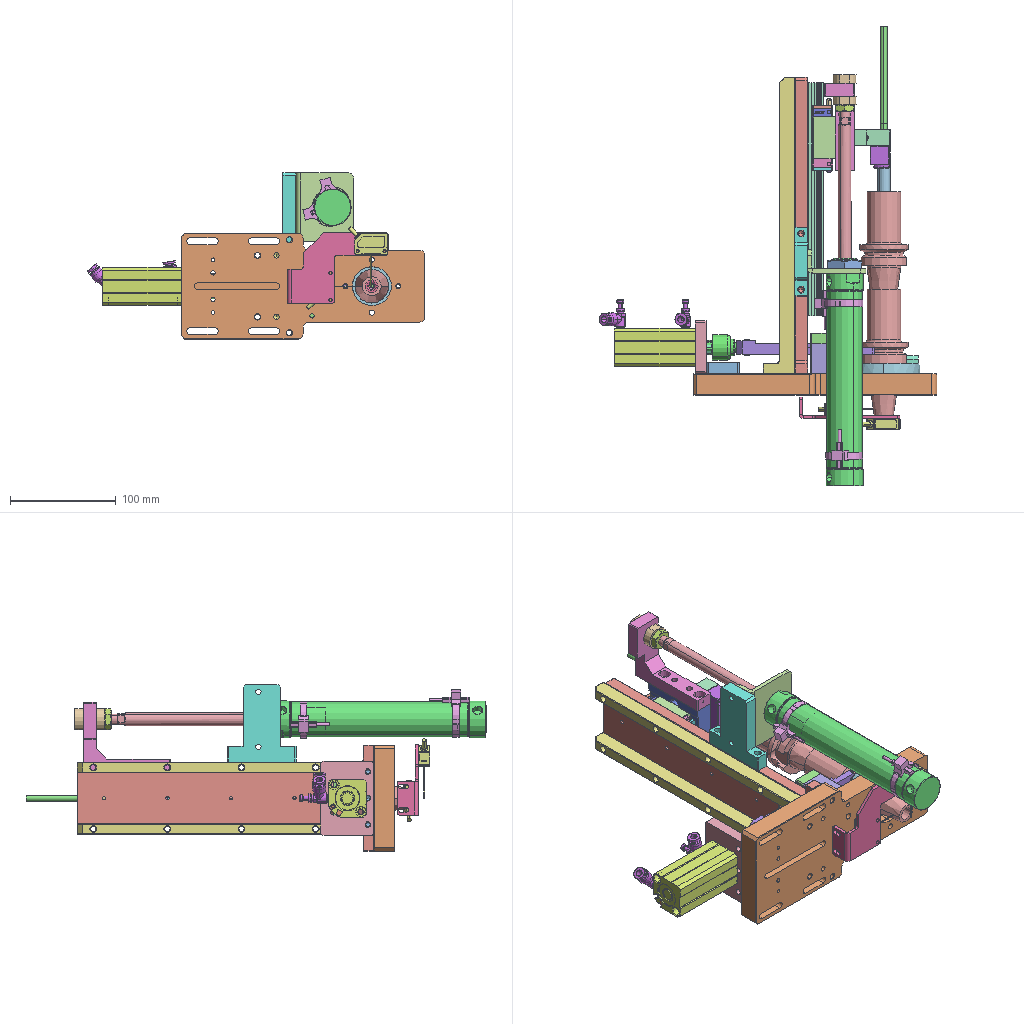Assembly | SolidWorks | 30 different items | 37 placed | box 319 x 435 x 157 mm
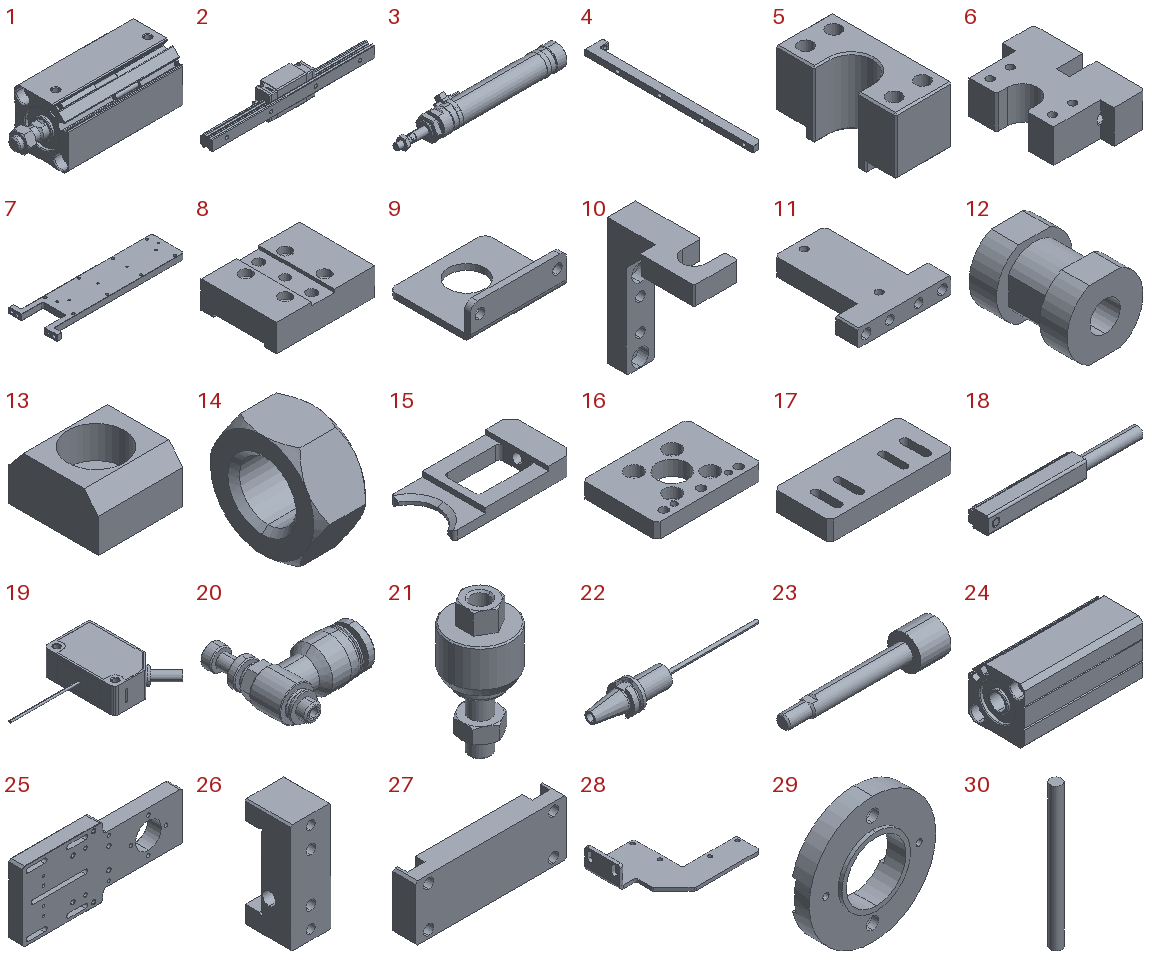Parts list (item | name | quantity | parent item | size | volume | features):
1 | (subassembly) | x1 | - | 95 x 36 x 36 mm | 77347 mm3 | -
2 | (subassembly) | x1 | - | 220 x 28 x 34 mm | 77398 mm3 | features AEMSimFeature 1
3 | (subassembly) | x1 | - | 263.352 x 41.739 x 46.528 mm | 110258 mm3 | features AEMSimFeature 1
4 | - | x2 | - | 30 x 280 x 10 mm | 40714 mm3 | features HoleWzd 3, Chamfer 2, Extrusion 1, Fillet 1, ICE 1
5 | - | x1 | - | 18 x 38 x 21 mm | 8331 mm3 | features Chamfer 1, Cut 1, Extrusion 1, HoleWzd 1, ICE 1
6 | - | x1 | - | 35 x 50 x 15 mm | 18159 mm3 | features HoleWzd 3, Chamfer 2, ICE 2, Cut 1, Extrusion 1
7 | - | x1 | - | 280 x 100 x 12 mm | 201479 mm3 | features HoleWzd 7, Chamfer 2, Fillet 2, Cut 1, Extrusion 1, ICE 1
8 | - | x1 | - | 65 x 50 x 18 mm | 47739 mm3 | features HoleWzd 6, Cut 3, Extrusion 1
9 | - | x1 | - | 65 x 55 x 22 mm | 16429 mm3 | features EdgeFlange 1, Fillet 1, FlatPattern 1, HoleWzd 1, ICE 1, SMBaseFlange 1, SheetMetal 1
10 | - | x1 | - | 28 x 65.5 x 82 mm | 28684 mm3 | features Chamfer 2, HoleWzd 2, ICE 2, Cut 1, Extrusion 1
11 | - | x1 | - | 65 x 73 x 12 mm | 33602 mm3 | features HoleWzd 3, Chamfer 2, Extrusion 1, ICE 1
12 | - | x1 | - | 22 x 28.5 x 20 mm | 6854 mm3 | features ICE 5, Extrusion 1, HoleWzd 1
13 | - | x2 | - | 15 x 15.8 x 9 mm | 1494 mm3 | features Extrusion 1, HoleWzd 1, ICE 1
14 | - | x1 | in 1 | 6 x 13.856 x 12.003 mm | 523.363 mm3 | features BaseBody 1
15 | - | x2 | - | 85 x 45 x 13 mm | 24143 mm3 | features ICE 6, Chamfer 3, Fillet 3, Extrusion 1, HoleWzd 1
16 | - | x1 | - | 70 x 50 x 10 mm | 27882 mm3 | features HoleWzd 3, Chamfer 1, Extrusion 1, ICE 1
17 | - | x1 | - | 70 x 32 x 11 mm | 21010 mm3 | features HoleWzd 4, Chamfer 1, Extrusion 1
18 | - | x2 | in 1 | 40.5 x 5.8 x 4.4 mm | 628.814 mm3 | features BaseBody 1
19 | - | x2 | - | 56.19 x 38.39 x 11 mm | 6633 mm3 | features BaseBody 1, ICE 1
20 | - | x2 | - | 28.5 x 30 x 12.5 mm | 2576 mm3 | features BaseBody 1
21 | - | x1 | - | 24 x 24 x 51 mm | 10568 mm3 | features BaseBody 1
22 | - | x2 | - | 277 x 46 x 46 mm | 91499 mm3 | features BaseBody 10
23 | - | x1 | in 1 | 91 x 20 x 20 mm | 10940 mm3 | features BaseBody 1
24 | - | x1 | in 1 | 76.5 x 36 x 36 mm | 64626 mm3 | features BaseBody 1
25 | - | x1 | - | 230 x 20 x 100 mm | 331110 mm3 | features HoleWzd 11, Chamfer 3, ICE 2, CirPattern 1, Cut 1, Extrusion 1, Fillet 1
26 | - | x1 | - | 25 x 28.4 x 68 mm | 31309 mm3 | features HoleWzd 3, ICE 2, Chamfer 1, Cut 1, Extrusion 1
27 | - | x1 | - | 68 x 10 x 25 mm | 15689 mm3 | features Chamfer 1, Extrusion 1, HoleWzd 1, ICE 1
28 | - | x1 | - | 95 x 67 x 20 mm | 11356 mm3 | features ICE 3, Chamfer 1, Cut 1, Fillet 1, FlatPattern 1, SMBaseFlange 1, SheetMetal 1
29 | - | x1 | - | 68 x 12 x 68 mm | 26017 mm3 | features ICE 6, HoleWzd 2, Revolution 1
30 | - | x1 | - | 12 x 12 x 150 mm | 16965 mm3 | features Extrusion 1
Mates (type | each side: item.copy, entity, surface, feature):
Coincident | 25.1 face plane Boss-Extrude 1 | 26.1 face plane Boss-Extrude 1
Coincident | 26.1 face plane Boss-Extrude 1 | 27.1 face plane Boss-Extrude 1 | 3 times
Symmetric | 25.1 face plane Boss-Extrude 1 | 25.1 face plane Boss-Extrude 1 | 26.1 plane
DistanceDim | 26.1 face plane Boss-Extrude 1 | 25.1 face plane Boss-Extrude 1
Coincident | 19.1 face plane E-MSMD61N-2M_l-1-solid1 | 28.1 face plane Base-Flange 1
Concentric | 19.1 face cylinder E-MSMD61N-2M_l-1-solid1 | 28.1 face cylinder Cut-Extrude 2 | 2 times
Coincident | 28.1 face plane Base-Flange 1 | 19.2 face plane E-MSMD61N-2M_l-1-solid1
Concentric | 28.1 face cylinder Cut-Extrude 2 | 19.2 face cylinder E-MSMD61N-2M_l-1-solid1 | 2 times
Coincident | 25.1 face plane Boss-Extrude 1 | 29.1 face plane Revolve 1
Concentric | 25.1 face cylinder Cut-Extrude 1 | 29.1 face cylinder Cut-Extrude 1
Coincident | 29.1 face plane Cut-Extrude 6 | 13.1 face plane Boss-Extrude 1
Concentric | 29.1 face cylinder M4 Tapped Hole 1 | 13.1 face cylinder M4 沉头Hole 1
Parallel | 29.1 face plane Cut-Extrude 6 | 13.1 face plane Boss-Extrude 1
Coincident | 29.1 face plane Cut-Extrude 6 | 13.2 face plane Boss-Extrude 1
Concentric | 29.1 face cylinder M4 Tapped Hole 1 | 13.2 face cylinder M4 沉头Hole 1
Parallel | 29.1 face plane Cut-Extrude 6 | 13.2 face plane Boss-Extrude 1
Concentric | 22.1 face cylinder BT30刀柄-0725-1-solid1 | 29.1 face cylinder Cut-Extrude 1
Coincident | 22.1 face plane BT30刀柄-0725-1-solid1 | 29.1 face plane Revolve 1
Concentric | 22.1 face cylinder BT30刀柄-0725-1-solid1 | 30.1 face cylinder Boss-Extrude 1
Coincident | 22.1 face plane BT30 Hole夹-1-solid1 | 30.1 face plane Boss-Extrude 1
Concentric | 25.1 face cylinder CirPattern 1 | 29.1 face cylinder M6 六角凹头Screw的柱形沉头Hole 1
Parallel | 22.1 face plane BT30刀柄-0725-1-solid1 | 13.1 face plane Boss-Extrude 1
Coincident | 5.1 face plane Boss-Extrude 1 | 6.1 face plane Boss-Extrude 1
Concentric | 5.1 face cylinder M4 六角凹头Screw的柱形沉头Hole 1 | 6.1 face cylinder M4 Tapped Hole 2 | 2 times
Width | 6.1 face plane Boss-Extrude 1 | 6.1 face plane Boss-Extrude 1 | 25.1 face plane Boss-Extrude 1 | 25.1 face plane Boss-Extrude 1
Concentric | 30.1 face cylinder Boss-Extrude 1 | 5.1 face cylinder Cut-Extrude 1
DistanceDim | 7.1 face plane Boss-Extrude 1 | 25.1 face plane Boss-Extrude 1
Width | 7.1 face plane Boss-Extrude 1 | 7.1 face plane Boss-Extrude 1 | 25.1 face plane Boss-Extrude 1 | 25.1 face plane Boss-Extrude 1
Coincident | 25.1 face plane Boss-Extrude 1 | 7.1 face plane Boss-Extrude 1
Coincident | 4.1 face plane Boss-Extrude 1 | 7.1 face plane Boss-Extrude 1 | 2 times
Coincident | 25.1 face plane Boss-Extrude 1 | 4.1 face plane Boss-Extrude 1
Coincident | 7.1 face plane Boss-Extrude 1 | 4.2 face plane Boss-Extrude 1 | 2 times
Coincident | 25.1 face plane Boss-Extrude 1 | 4.2 face plane Boss-Extrude 1
Symmetric | 7.1 face plane Boss-Extrude 1 | 7.1 face plane Boss-Extrude 1 | 2.1 plane
Concentric | 22.1 face cylinder BT30刀柄-0725-1-solid1 | 22.2 face cylinder BT30刀柄-0725-1-solid1
Parallel | 22.1 face plane BT30刀柄-0725-1-solid1 | 22.2 face plane BT30刀柄-0725-1-solid1
DistanceDim | 22.1 face plane BT30刀柄-0725-1-solid1 | 22.2 face plane BT30刀柄-0725-1-solid1
Coincident | 8.1 face plane Boss-Extrude 1 | 10.1 face plane Boss-Extrude 1 | 2 times
Coincident | 7.1 face plane Boss-Extrude 1 | 9.1 face plane Edge-Flange 1
DistanceDim | 9.1 face plane Base-Flange 1 | 7.1 face plane Boss-Extrude 1
DistanceDim | 9.1 face plane Base-Flange 1 | 25.1 face plane Boss-Extrude 1
Coincident | 8.1 face plane Boss-Extrude 1 | 10.1 face plane Boss-Extrude 3
Coincident | 7.1 face plane Boss-Extrude 1 | 11.1 face plane Boss-Extrude 1 | 2 times
Width | 11.1 face plane Boss-Extrude 1 | 11.1 face plane Boss-Extrude 1 | 9.1 face plane Edge-Flange 1 | 9.1 face plane Base-Flange 1
DistanceDim | 28.1 face plane Base-Flange 1 | 25.1 face plane Boss-Extrude 1 | 3 times
Width | 12.1 face plane Boss-Extrude 1 | 12.1 face plane Boss-Extrude 3 | 10.1 face plane Boss-Extrude 1 | 10.1 face plane Boss-Extrude 1
Parallel | 25.1 face plane Boss-Extrude 1 | 15.1 face plane Boss-Extrude 1
Coincident | 15.1 face plane Boss-Extrude 1 | 15.2 face plane Boss-Extrude 1 | 2 times
Concentric | 22.1 face cylinder BT30刀柄-0725-1-solid1 | 15.2 face cylinder Cut-Extrude 3
Coincident | 15.1 face plane Boss-Extrude 1 | 21.1 face plane 输入1
Concentric | 15.1 face cylinder M8 Tapped Hole 1 | 21.1 face cylinder 输入1
DistanceDim | 15.2 face plane Boss-Extrude 1 | 15.1 face plane Boss-Extrude 1
Coincident | 25.1 face plane Boss-Extrude 1 | 17.1 face plane Boss-Extrude 1
Coincident | 16.1 face plane Boss-Extrude 1 | 17.1 face plane Boss-Extrude 1 | 2 times
Concentric | 16.1 face cylinder Cut-Extrude 1 | 23.1 face cone 输入1
Coincident | 16.1 face plane Boss-Extrude 1 | 24.1 face plane 输入1
Coincident | 25.1 face plane Boss-Extrude 1 | 16.1 face plane Boss-Extrude 1
Width | 17.1 face plane Boss-Extrude 1 | 17.1 face plane Boss-Extrude 1 | 25.1 face plane Boss-Extrude 1 | 25.1 face plane Boss-Extrude 1
DistanceDim | 16.1 face plane Boss-Extrude 1 | 25.1 face plane Boss-Extrude 1
Concentric | 21.1 face cylinder 输入1 | 23.1 face cylinder 输入1
Concentric | 16.1 face cylinder M6 六角圆柱头Screw的柱形沉头Hole 1 | 24.1 face cylinder 输入1
Concentric | 20.1 face cylinder 输入1 | 24.1 face cylinder 输入1
Coincident | 20.1 face plane 输入1 | 24.1 face plane 输入1
Concentric | 20.2 face cylinder 输入1 | 24.1 face cylinder 输入1
Coincident | 20.2 face plane 输入1 | 24.1 face plane 输入1